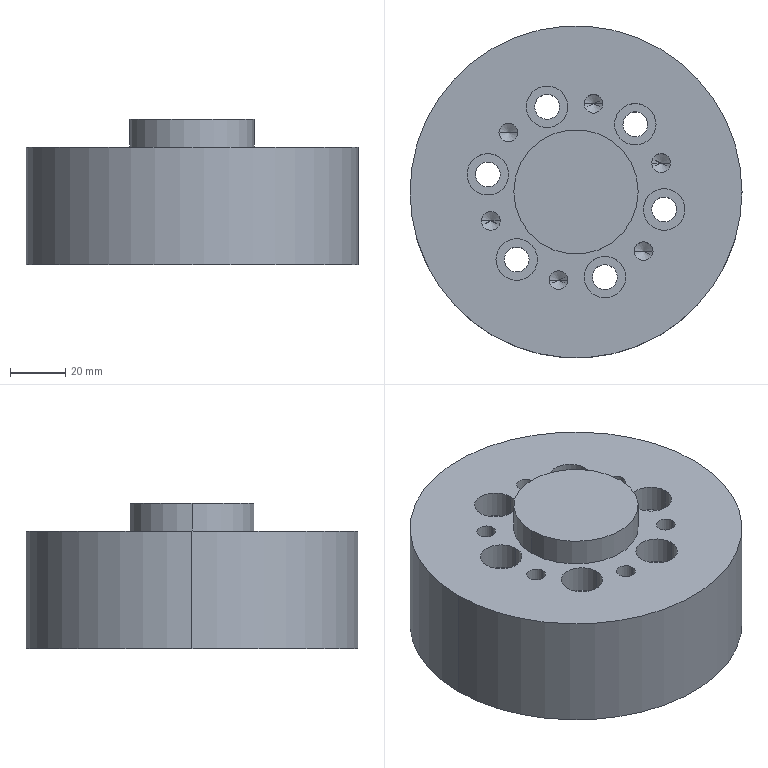Part | 1 solid | 64 faces | box 120 x 120 x 52.5 mm | volume 443606 mm3 | cylinder 42 | cone 12 | plane 10 | commonest cylinder face diameters 6.8 x12 9 x12 15 x12 45 x4 120 x2